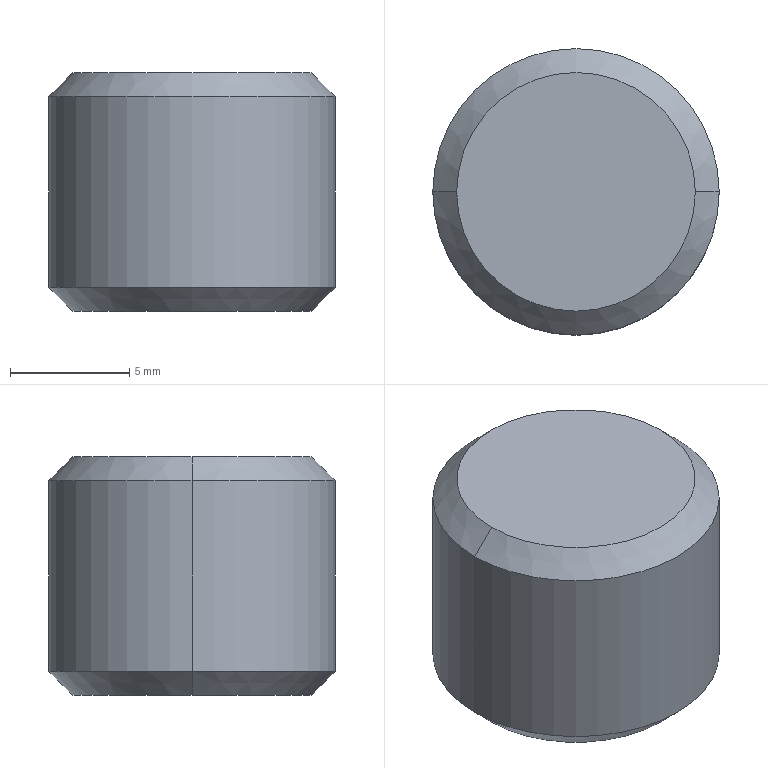Part | SolidWorks | features BaseBody 1 | 1 solid | 8 faces | box 12.005 x 12.005 x 10 mm | volume 1096 mm3 | cone 4 | cylinder 2 | plane 2 | commonest cylinder face diameters 12.005 x2
STEP:
#1=CARTESIAN_POINT('',(-91.002,-25.,-43.829));
#2=VERTEX_POINT('',#1);
#3=CARTESIAN_POINT('',(-80.998,-25.,-43.829));
#4=VERTEX_POINT('',#3);
#5=CARTESIAN_POINT('',(-86.,-25.,-43.829));
#6=DIRECTION('',(0.,0.,-1.));
#7=DIRECTION('',(-1.,0.,0.));
#8=AXIS2_PLACEMENT_3D('',#5,#6,#7);
#9=CIRCLE('',#8,5.002);
#10=EDGE_CURVE('',#2,#4,#9,.T.);
#11=ORIENTED_EDGE('',*,*,#10,.F.);
#12=CARTESIAN_POINT('',(-92.002,-25.,-42.829));
#13=VERTEX_POINT('',#12);
#14=CARTESIAN_POINT('',(-92.002,-25.,-42.829));
#15=DIRECTION('',(-0.7071,0.,0.7071));
#16=VECTOR('',#15,1000.);
#17=LINE('',#14,#16);
#18=EDGE_CURVE('',#2,#13,#17,.T.);
#19=ORIENTED_EDGE('',*,*,#18,.T.);
#20=CARTESIAN_POINT('',(-79.998,-25.,-42.829));
#21=VERTEX_POINT('',#20);
#22=CARTESIAN_POINT('',(-86.,-25.,-42.829));
#23=DIRECTION('',(0.,0.,1.));
#24=DIRECTION('',(-1.,0.,0.));
#25=AXIS2_PLACEMENT_3D('',#22,#23,#24);
#26=CIRCLE('',#25,6.002);
#27=EDGE_CURVE('',#21,#13,#26,.T.);
#28=ORIENTED_EDGE('',*,*,#27,.F.);
#29=CARTESIAN_POINT('',(-79.998,-25.,-42.829));
#30=DIRECTION('',(0.7071,0.,0.7071));
#31=VECTOR('',#30,1000.);
#32=LINE('',#29,#31);
#33=EDGE_CURVE('',#4,#21,#32,.T.);
#34=ORIENTED_EDGE('',*,*,#33,.F.);
#35=EDGE_LOOP('',(#11,#19,#28,#34));
#36=FACE_OUTER_BOUND('',#35,.T.);
#37=CARTESIAN_POINT('',(-86.,-25.,-42.829));
#38=DIRECTION('',(0.,0.,1.));
#39=DIRECTION('',(1.,0.,0.));
#40=AXIS2_PLACEMENT_3D('',#37,#38,#39);
#41=CONICAL_SURFACE('',#40,6.002,0.7854);
#42=ADVANCED_FACE('',(#36),#41,.T.);
#43=CARTESIAN_POINT('',(-80.998,-25.,-33.829));
#44=VERTEX_POINT('',#43);
#45=CARTESIAN_POINT('',(-91.002,-25.,-33.829));
#46=VERTEX_POINT('',#45);
#47=CARTESIAN_POINT('',(-86.,-25.,-33.829));
#48=DIRECTION('',(0.,0.,1.));
#49=DIRECTION('',(1.,0.,0.));
#50=AXIS2_PLACEMENT_3D('',#47,#48,#49);
#51=CIRCLE('',#50,5.002);
#52=EDGE_CURVE('',#44,#46,#51,.T.);
#53=ORIENTED_EDGE('',*,*,#52,.F.);
#54=CARTESIAN_POINT('',(-79.998,-25.,-34.829));
#55=VERTEX_POINT('',#54);
#56=CARTESIAN_POINT('',(-79.998,-25.,-34.829));
#57=DIRECTION('',(0.7071,0.,-0.7071));
#58=VECTOR('',#57,1000.);
#59=LINE('',#56,#58);
#60=EDGE_CURVE('',#44,#55,#59,.T.);
#61=ORIENTED_EDGE('',*,*,#60,.T.);
#62=CARTESIAN_POINT('',(-92.002,-25.,-34.829));
#63=VERTEX_POINT('',#62);
#64=CARTESIAN_POINT('',(-86.,-25.,-34.829));
#65=DIRECTION('',(0.,0.,-1.));
#66=DIRECTION('',(1.,0.,0.));
#67=AXIS2_PLACEMENT_3D('',#64,#65,#66);
#68=CIRCLE('',#67,6.002);
#69=EDGE_CURVE('',#63,#55,#68,.T.);
#70=ORIENTED_EDGE('',*,*,#69,.F.);
#71=CARTESIAN_POINT('',(-92.002,-25.,-34.829));
#72=DIRECTION('',(-0.7071,0.,-0.7071));
#73=VECTOR('',#72,1000.);
#74=LINE('',#71,#73);
#75=EDGE_CURVE('',#46,#63,#74,.T.);
#76=ORIENTED_EDGE('',*,*,#75,.F.);
#77=EDGE_LOOP('',(#53,#61,#70,#76));
#78=FACE_OUTER_BOUND('',#77,.T.);
#79=CARTESIAN_POINT('',(-86.,-25.,-34.829));
#80=DIRECTION('',(0.,0.,-1.));
#81=DIRECTION('',(-1.,0.,0.));
#82=AXIS2_PLACEMENT_3D('',#79,#80,#81);
#83=CONICAL_SURFACE('',#82,6.002,0.7854);
#84=ADVANCED_FACE('',(#78),#83,.T.);
#85=CARTESIAN_POINT('',(-86.,-25.,-34.829));
#86=DIRECTION('',(0.,0.,-1.));
#87=DIRECTION('',(1.,0.,0.));
#88=AXIS2_PLACEMENT_3D('',#85,#86,#87);
#89=CIRCLE('',#88,6.002);
#90=EDGE_CURVE('',#55,#63,#89,.T.);
#91=ORIENTED_EDGE('',*,*,#90,.T.);
#92=CARTESIAN_POINT('',(-92.002,-25.,-33.829));
#93=DIRECTION('',(0.,0.,-1.));
#94=VECTOR('',#93,1000.);
#95=LINE('',#92,#94);
#96=EDGE_CURVE('',#63,#13,#95,.T.);
#97=ORIENTED_EDGE('',*,*,#96,.T.);
#98=CARTESIAN_POINT('',(-86.,-25.,-42.829));
#99=DIRECTION('',(0.,0.,1.));
#100=DIRECTION('',(-1.,0.,0.));
#101=AXIS2_PLACEMENT_3D('',#98,#99,#100);
#102=CIRCLE('',#101,6.002);
#103=EDGE_CURVE('',#13,#21,#102,.T.);
#104=ORIENTED_EDGE('',*,*,#103,.T.);
#105=CARTESIAN_POINT('',(-79.998,-25.,-33.829));
#106=DIRECTION('',(0.,0.,-1.));
#107=VECTOR('',#106,1000.);
#108=LINE('',#105,#107);
#109=EDGE_CURVE('',#55,#21,#108,.T.);
#110=ORIENTED_EDGE('',*,*,#109,.F.);
#111=EDGE_LOOP('',(#91,#97,#104,#110));
#112=FACE_OUTER_BOUND('',#111,.T.);
#113=CARTESIAN_POINT('',(-86.,-25.,-33.829));
#114=DIRECTION('',(0.,0.,-1.));
#115=DIRECTION('',(1.,0.,0.));
#116=AXIS2_PLACEMENT_3D('',#113,#114,#115);
#117=CYLINDRICAL_SURFACE('',#116,6.002);
#118=ADVANCED_FACE('',(#112),#117,.T.);
#119=CARTESIAN_POINT('',(-86.,-25.,-43.829));
#120=DIRECTION('',(0.,0.,-1.));
#121=DIRECTION('',(-1.,0.,0.));
#122=AXIS2_PLACEMENT_3D('',#119,#120,#121);
#123=CIRCLE('',#122,5.002);
#124=EDGE_CURVE('',#4,#2,#123,.T.);
#125=ORIENTED_EDGE('',*,*,#124,.T.);
#126=ORIENTED_EDGE('',*,*,#10,.T.);
#127=EDGE_LOOP('',(#125,#126));
#128=FACE_OUTER_BOUND('',#127,.T.);
#129=CARTESIAN_POINT('',(-86.,-25.,-43.829));
#130=DIRECTION('',(0.,0.,-1.));
#131=DIRECTION('',(-1.,0.,0.));
#132=AXIS2_PLACEMENT_3D('',#129,#130,#131);
#133=PLANE('',#132);
#134=ADVANCED_FACE('',(#128),#133,.T.);
#135=CARTESIAN_POINT('',(-86.,-25.,-33.829));
#136=DIRECTION('',(0.,0.,1.));
#137=DIRECTION('',(1.,0.,0.));
#138=AXIS2_PLACEMENT_3D('',#135,#136,#137);
#139=CIRCLE('',#138,5.002);
#140=EDGE_CURVE('',#46,#44,#139,.T.);
#141=ORIENTED_EDGE('',*,*,#140,.T.);
#142=ORIENTED_EDGE('',*,*,#52,.T.);
#143=EDGE_LOOP('',(#141,#142));
#144=FACE_OUTER_BOUND('',#143,.T.);
#145=CARTESIAN_POINT('',(-86.,-25.,-33.829));
#146=DIRECTION('',(0.,0.,1.));
#147=DIRECTION('',(1.,0.,0.));
#148=AXIS2_PLACEMENT_3D('',#145,#146,#147);
#149=PLANE('',#148);
#150=ADVANCED_FACE('',(#144),#149,.T.);
#151=ORIENTED_EDGE('',*,*,#96,.F.);
#152=ORIENTED_EDGE('',*,*,#69,.T.);
#153=ORIENTED_EDGE('',*,*,#109,.T.);
#154=ORIENTED_EDGE('',*,*,#27,.T.);
#155=EDGE_LOOP('',(#151,#152,#153,#154));
#156=FACE_OUTER_BOUND('',#155,.T.);
#157=CARTESIAN_POINT('',(-86.,-25.,-33.829));
#158=DIRECTION('',(0.,0.,-1.));
#159=DIRECTION('',(1.,0.,0.));
#160=AXIS2_PLACEMENT_3D('',#157,#158,#159);
#161=CYLINDRICAL_SURFACE('',#160,6.002);
#162=ADVANCED_FACE('',(#156),#161,.T.);
#163=ORIENTED_EDGE('',*,*,#60,.F.);
#164=ORIENTED_EDGE('',*,*,#140,.F.);
#165=ORIENTED_EDGE('',*,*,#75,.T.);
#166=ORIENTED_EDGE('',*,*,#90,.F.);
#167=EDGE_LOOP('',(#163,#164,#165,#166));
#168=FACE_OUTER_BOUND('',#167,.T.);
#169=CARTESIAN_POINT('',(-86.,-25.,-34.829));
#170=DIRECTION('',(0.,0.,-1.));
#171=DIRECTION('',(-1.,0.,0.));
#172=AXIS2_PLACEMENT_3D('',#169,#170,#171);
#173=CONICAL_SURFACE('',#172,6.002,0.7854);
#174=ADVANCED_FACE('',(#168),#173,.T.);
#175=ORIENTED_EDGE('',*,*,#18,.F.);
#176=ORIENTED_EDGE('',*,*,#124,.F.);
#177=ORIENTED_EDGE('',*,*,#33,.T.);
#178=ORIENTED_EDGE('',*,*,#103,.F.);
#179=EDGE_LOOP('',(#175,#176,#177,#178));
#180=FACE_OUTER_BOUND('',#179,.T.);
#181=CARTESIAN_POINT('',(-86.,-25.,-42.829));
#182=DIRECTION('',(0.,0.,1.));
#183=DIRECTION('',(1.,0.,0.));
#184=AXIS2_PLACEMENT_3D('',#181,#182,#183);
#185=CONICAL_SURFACE('',#184,6.002,0.7854);
#186=ADVANCED_FACE('',(#180),#185,.T.);
#187=CLOSED_SHELL('',(#42,#84,#118,#134,#150,#162,#174,#186));
#188=MANIFOLD_SOLID_BREP('',#187);
#189=CARTESIAN_POINT('',(0.,0.,0.));
#190=DIRECTION('',(0.,0.,1.));
#191=DIRECTION('',(1.,0.,0.));
#192=AXIS2_PLACEMENT_3D('',#189,#190,#191);
#193=(LENGTH_UNIT()NAMED_UNIT(*)SI_UNIT(.MILLI.,.METRE.));
#194=UNCERTAINTY_MEASURE_WITH_UNIT(LENGTH_MEASURE(0.00001),#193,'','');
#195=(NAMED_UNIT(*)PLANE_ANGLE_UNIT()SI_UNIT($,.RADIAN.));
#196=(NAMED_UNIT(*)SI_UNIT($,.STERADIAN.)SOLID_ANGLE_UNIT());
#197=(GEOMETRIC_REPRESENTATION_CONTEXT(3)GLOBAL_UNCERTAINTY_ASSIGNED_CONTEXT((#194))GLOBAL_UNIT_ASSIGNED_CONTEXT((#193,#195,#196))REPRESENTATION_CONTEXT('',''));
#198=ADVANCED_BREP_SHAPE_REPRESENTATION('',(#188,#192),#197);